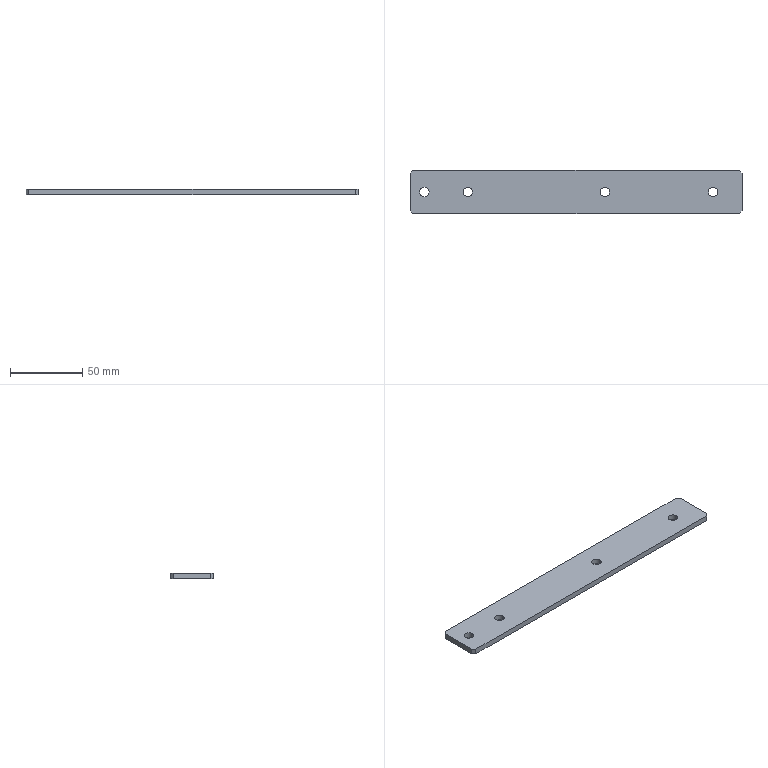Part | SolidWorks | features Chamfer 1, Extrusion 1 | 1 solid | 18 faces | box 230 x 30 x 4 mm | volume 27037 mm3 | plane 10 | cylinder 8 | commonest cylinder face diameters 6.5 x8
STEP:
#1=CARTESIAN_POINT('',(91.75,0.,4.));
#2=VERTEX_POINT('',#1);
#3=CARTESIAN_POINT('',(98.25,0.,4.));
#4=VERTEX_POINT('',#3);
#5=CARTESIAN_POINT('',(95.,0.,4.));
#6=DIRECTION('',(0.,0.,1.));
#7=DIRECTION('',(1.,0.,0.));
#8=AXIS2_PLACEMENT_3D('',#5,#6,#7);
#9=CIRCLE('',#8,3.25);
#10=EDGE_CURVE('',#2,#4,#9,.T.);
#11=ORIENTED_EDGE('',*,*,#10,.T.);
#12=CARTESIAN_POINT('',(98.25,0.,0.));
#13=VERTEX_POINT('',#12);
#14=CARTESIAN_POINT('',(98.25,0.,4.));
#15=DIRECTION('',(0.,0.,-1.));
#16=VECTOR('',#15,1000.);
#17=LINE('',#14,#16);
#18=EDGE_CURVE('',#4,#13,#17,.T.);
#19=ORIENTED_EDGE('',*,*,#18,.T.);
#20=CARTESIAN_POINT('',(91.75,0.,0.));
#21=VERTEX_POINT('',#20);
#22=CARTESIAN_POINT('',(95.,0.,0.));
#23=DIRECTION('',(0.,0.,1.));
#24=DIRECTION('',(1.,0.,0.));
#25=AXIS2_PLACEMENT_3D('',#22,#23,#24);
#26=CIRCLE('',#25,3.25);
#27=EDGE_CURVE('',#21,#13,#26,.T.);
#28=ORIENTED_EDGE('',*,*,#27,.F.);
#29=CARTESIAN_POINT('',(91.75,0.,4.));
#30=DIRECTION('',(0.,0.,-1.));
#31=VECTOR('',#30,1000.);
#32=LINE('',#29,#31);
#33=EDGE_CURVE('',#2,#21,#32,.T.);
#34=ORIENTED_EDGE('',*,*,#33,.F.);
#35=EDGE_LOOP('',(#11,#19,#28,#34));
#36=FACE_OUTER_BOUND('',#35,.T.);
#37=CARTESIAN_POINT('',(95.,0.,4.));
#38=DIRECTION('',(0.,0.,-1.));
#39=DIRECTION('',(-1.,0.,0.));
#40=AXIS2_PLACEMENT_3D('',#37,#38,#39);
#41=CYLINDRICAL_SURFACE('',#40,3.25);
#42=ADVANCED_FACE('',(#36),#41,.F.);
#43=CARTESIAN_POINT('',(16.75,0.,4.));
#44=VERTEX_POINT('',#43);
#45=CARTESIAN_POINT('',(23.25,0.,4.));
#46=VERTEX_POINT('',#45);
#47=CARTESIAN_POINT('',(20.,0.,4.));
#48=DIRECTION('',(0.,0.,1.));
#49=DIRECTION('',(1.,0.,0.));
#50=AXIS2_PLACEMENT_3D('',#47,#48,#49);
#51=CIRCLE('',#50,3.25);
#52=EDGE_CURVE('',#44,#46,#51,.T.);
#53=ORIENTED_EDGE('',*,*,#52,.T.);
#54=CARTESIAN_POINT('',(23.25,0.,0.));
#55=VERTEX_POINT('',#54);
#56=CARTESIAN_POINT('',(23.25,0.,4.));
#57=DIRECTION('',(0.,0.,-1.));
#58=VECTOR('',#57,1000.);
#59=LINE('',#56,#58);
#60=EDGE_CURVE('',#46,#55,#59,.T.);
#61=ORIENTED_EDGE('',*,*,#60,.T.);
#62=CARTESIAN_POINT('',(16.75,0.,0.));
#63=VERTEX_POINT('',#62);
#64=CARTESIAN_POINT('',(20.,0.,0.));
#65=DIRECTION('',(0.,0.,1.));
#66=DIRECTION('',(1.,0.,0.));
#67=AXIS2_PLACEMENT_3D('',#64,#65,#66);
#68=CIRCLE('',#67,3.25);
#69=EDGE_CURVE('',#63,#55,#68,.T.);
#70=ORIENTED_EDGE('',*,*,#69,.F.);
#71=CARTESIAN_POINT('',(16.75,0.,4.));
#72=DIRECTION('',(0.,0.,-1.));
#73=VECTOR('',#72,1000.);
#74=LINE('',#71,#73);
#75=EDGE_CURVE('',#44,#63,#74,.T.);
#76=ORIENTED_EDGE('',*,*,#75,.F.);
#77=EDGE_LOOP('',(#53,#61,#70,#76));
#78=FACE_OUTER_BOUND('',#77,.T.);
#79=CARTESIAN_POINT('',(20.,0.,4.));
#80=DIRECTION('',(0.,0.,-1.));
#81=DIRECTION('',(-1.,0.,0.));
#82=AXIS2_PLACEMENT_3D('',#79,#80,#81);
#83=CYLINDRICAL_SURFACE('',#82,3.25);
#84=ADVANCED_FACE('',(#78),#83,.F.);
#85=CARTESIAN_POINT('',(-78.25,0.,4.));
#86=VERTEX_POINT('',#85);
#87=CARTESIAN_POINT('',(-71.75,0.,4.));
#88=VERTEX_POINT('',#87);
#89=CARTESIAN_POINT('',(-75.,0.,4.));
#90=DIRECTION('',(0.,0.,1.));
#91=DIRECTION('',(1.,0.,0.));
#92=AXIS2_PLACEMENT_3D('',#89,#90,#91);
#93=CIRCLE('',#92,3.25);
#94=EDGE_CURVE('',#86,#88,#93,.T.);
#95=ORIENTED_EDGE('',*,*,#94,.T.);
#96=CARTESIAN_POINT('',(-71.75,0.,0.));
#97=VERTEX_POINT('',#96);
#98=CARTESIAN_POINT('',(-71.75,0.,4.));
#99=DIRECTION('',(0.,0.,-1.));
#100=VECTOR('',#99,1000.);
#101=LINE('',#98,#100);
#102=EDGE_CURVE('',#88,#97,#101,.T.);
#103=ORIENTED_EDGE('',*,*,#102,.T.);
#104=CARTESIAN_POINT('',(-78.25,0.,0.));
#105=VERTEX_POINT('',#104);
#106=CARTESIAN_POINT('',(-75.,0.,0.));
#107=DIRECTION('',(0.,0.,1.));
#108=DIRECTION('',(1.,0.,0.));
#109=AXIS2_PLACEMENT_3D('',#106,#107,#108);
#110=CIRCLE('',#109,3.25);
#111=EDGE_CURVE('',#105,#97,#110,.T.);
#112=ORIENTED_EDGE('',*,*,#111,.F.);
#113=CARTESIAN_POINT('',(-78.25,0.,4.));
#114=DIRECTION('',(0.,0.,-1.));
#115=VECTOR('',#114,1000.);
#116=LINE('',#113,#115);
#117=EDGE_CURVE('',#86,#105,#116,.T.);
#118=ORIENTED_EDGE('',*,*,#117,.F.);
#119=EDGE_LOOP('',(#95,#103,#112,#118));
#120=FACE_OUTER_BOUND('',#119,.T.);
#121=CARTESIAN_POINT('',(-75.,0.,4.));
#122=DIRECTION('',(0.,0.,-1.));
#123=DIRECTION('',(-1.,0.,0.));
#124=AXIS2_PLACEMENT_3D('',#121,#122,#123);
#125=CYLINDRICAL_SURFACE('',#124,3.25);
#126=ADVANCED_FACE('',(#120),#125,.F.);
#127=CARTESIAN_POINT('',(-108.25,0.,4.));
#128=VERTEX_POINT('',#127);
#129=CARTESIAN_POINT('',(-101.75,0.,4.));
#130=VERTEX_POINT('',#129);
#131=CARTESIAN_POINT('',(-105.,0.,4.));
#132=DIRECTION('',(0.,0.,1.));
#133=DIRECTION('',(1.,0.,0.));
#134=AXIS2_PLACEMENT_3D('',#131,#132,#133);
#135=CIRCLE('',#134,3.25);
#136=EDGE_CURVE('',#128,#130,#135,.T.);
#137=ORIENTED_EDGE('',*,*,#136,.T.);
#138=CARTESIAN_POINT('',(-101.75,0.,0.));
#139=VERTEX_POINT('',#138);
#140=CARTESIAN_POINT('',(-101.75,0.,4.));
#141=DIRECTION('',(0.,0.,-1.));
#142=VECTOR('',#141,1000.);
#143=LINE('',#140,#142);
#144=EDGE_CURVE('',#130,#139,#143,.T.);
#145=ORIENTED_EDGE('',*,*,#144,.T.);
#146=CARTESIAN_POINT('',(-108.25,0.,0.));
#147=VERTEX_POINT('',#146);
#148=CARTESIAN_POINT('',(-105.,0.,0.));
#149=DIRECTION('',(0.,0.,1.));
#150=DIRECTION('',(1.,0.,0.));
#151=AXIS2_PLACEMENT_3D('',#148,#149,#150);
#152=CIRCLE('',#151,3.25);
#153=EDGE_CURVE('',#147,#139,#152,.T.);
#154=ORIENTED_EDGE('',*,*,#153,.F.);
#155=CARTESIAN_POINT('',(-108.25,0.,4.));
#156=DIRECTION('',(0.,0.,-1.));
#157=VECTOR('',#156,1000.);
#158=LINE('',#155,#157);
#159=EDGE_CURVE('',#128,#147,#158,.T.);
#160=ORIENTED_EDGE('',*,*,#159,.F.);
#161=EDGE_LOOP('',(#137,#145,#154,#160));
#162=FACE_OUTER_BOUND('',#161,.T.);
#163=CARTESIAN_POINT('',(-105.,0.,4.));
#164=DIRECTION('',(0.,0.,-1.));
#165=DIRECTION('',(-1.,0.,0.));
#166=AXIS2_PLACEMENT_3D('',#163,#164,#165);
#167=CYLINDRICAL_SURFACE('',#166,3.25);
#168=ADVANCED_FACE('',(#162),#167,.F.);
#169=CARTESIAN_POINT('',(-115.,13.,4.));
#170=VERTEX_POINT('',#169);
#171=CARTESIAN_POINT('',(-115.,-13.,4.));
#172=VERTEX_POINT('',#171);
#173=CARTESIAN_POINT('',(-115.,15.,4.));
#174=DIRECTION('',(0.,-1.,0.));
#175=VECTOR('',#174,1000.);
#176=LINE('',#173,#175);
#177=EDGE_CURVE('',#170,#172,#176,.T.);
#178=ORIENTED_EDGE('',*,*,#177,.T.);
#179=CARTESIAN_POINT('',(-113.,-15.,4.));
#180=VERTEX_POINT('',#179);
#181=CARTESIAN_POINT('',(-113.,-15.,4.));
#182=DIRECTION('',(0.7071,-0.7071,0.));
#183=VECTOR('',#182,1000.);
#184=LINE('',#181,#183);
#185=EDGE_CURVE('',#172,#180,#184,.T.);
#186=ORIENTED_EDGE('',*,*,#185,.T.);
#187=CARTESIAN_POINT('',(113.,-15.,4.));
#188=VERTEX_POINT('',#187);
#189=CARTESIAN_POINT('',(115.,-15.,4.));
#190=DIRECTION('',(1.,0.,0.));
#191=VECTOR('',#190,1000.);
#192=LINE('',#189,#191);
#193=EDGE_CURVE('',#180,#188,#192,.T.);
#194=ORIENTED_EDGE('',*,*,#193,.T.);
#195=CARTESIAN_POINT('',(115.,-13.,4.));
#196=VERTEX_POINT('',#195);
#197=CARTESIAN_POINT('',(115.,-13.,4.));
#198=DIRECTION('',(0.7071,0.7071,0.));
#199=VECTOR('',#198,1000.);
#200=LINE('',#197,#199);
#201=EDGE_CURVE('',#188,#196,#200,.T.);
#202=ORIENTED_EDGE('',*,*,#201,.T.);
#203=CARTESIAN_POINT('',(115.,13.,4.));
#204=VERTEX_POINT('',#203);
#205=CARTESIAN_POINT('',(115.,15.,4.));
#206=DIRECTION('',(0.,1.,0.));
#207=VECTOR('',#206,1000.);
#208=LINE('',#205,#207);
#209=EDGE_CURVE('',#196,#204,#208,.T.);
#210=ORIENTED_EDGE('',*,*,#209,.T.);
#211=CARTESIAN_POINT('',(113.,15.,4.));
#212=VERTEX_POINT('',#211);
#213=CARTESIAN_POINT('',(113.,15.,4.));
#214=DIRECTION('',(-0.7071,0.7071,0.));
#215=VECTOR('',#214,1000.);
#216=LINE('',#213,#215);
#217=EDGE_CURVE('',#204,#212,#216,.T.);
#218=ORIENTED_EDGE('',*,*,#217,.T.);
#219=CARTESIAN_POINT('',(-113.,15.,4.));
#220=VERTEX_POINT('',#219);
#221=CARTESIAN_POINT('',(115.,15.,4.));
#222=DIRECTION('',(-1.,0.,0.));
#223=VECTOR('',#222,1000.);
#224=LINE('',#221,#223);
#225=EDGE_CURVE('',#212,#220,#224,.T.);
#226=ORIENTED_EDGE('',*,*,#225,.T.);
#227=CARTESIAN_POINT('',(-115.,13.,4.));
#228=DIRECTION('',(-0.7071,-0.7071,0.));
#229=VECTOR('',#228,1000.);
#230=LINE('',#227,#229);
#231=EDGE_CURVE('',#220,#170,#230,.T.);
#232=ORIENTED_EDGE('',*,*,#231,.T.);
#233=EDGE_LOOP('',(#178,#186,#194,#202,#210,#218,#226,#232));
#234=FACE_OUTER_BOUND('',#233,.T.);
#235=ORIENTED_EDGE('',*,*,#136,.F.);
#236=CARTESIAN_POINT('',(-105.,0.,4.));
#237=DIRECTION('',(0.,0.,1.));
#238=DIRECTION('',(1.,0.,0.));
#239=AXIS2_PLACEMENT_3D('',#236,#237,#238);
#240=CIRCLE('',#239,3.25);
#241=EDGE_CURVE('',#130,#128,#240,.T.);
#242=ORIENTED_EDGE('',*,*,#241,.F.);
#243=EDGE_LOOP('',(#235,#242));
#244=FACE_BOUND('',#243,.T.);
#245=ORIENTED_EDGE('',*,*,#94,.F.);
#246=CARTESIAN_POINT('',(-75.,0.,4.));
#247=DIRECTION('',(0.,0.,1.));
#248=DIRECTION('',(1.,0.,0.));
#249=AXIS2_PLACEMENT_3D('',#246,#247,#248);
#250=CIRCLE('',#249,3.25);
#251=EDGE_CURVE('',#88,#86,#250,.T.);
#252=ORIENTED_EDGE('',*,*,#251,.F.);
#253=EDGE_LOOP('',(#245,#252));
#254=FACE_BOUND('',#253,.T.);
#255=ORIENTED_EDGE('',*,*,#52,.F.);
#256=CARTESIAN_POINT('',(20.,0.,4.));
#257=DIRECTION('',(0.,0.,1.));
#258=DIRECTION('',(1.,0.,0.));
#259=AXIS2_PLACEMENT_3D('',#256,#257,#258);
#260=CIRCLE('',#259,3.25);
#261=EDGE_CURVE('',#46,#44,#260,.T.);
#262=ORIENTED_EDGE('',*,*,#261,.F.);
#263=EDGE_LOOP('',(#255,#262));
#264=FACE_BOUND('',#263,.T.);
#265=ORIENTED_EDGE('',*,*,#10,.F.);
#266=CARTESIAN_POINT('',(95.,0.,4.));
#267=DIRECTION('',(0.,0.,1.));
#268=DIRECTION('',(1.,0.,0.));
#269=AXIS2_PLACEMENT_3D('',#266,#267,#268);
#270=CIRCLE('',#269,3.25);
#271=EDGE_CURVE('',#4,#2,#270,.T.);
#272=ORIENTED_EDGE('',*,*,#271,.F.);
#273=EDGE_LOOP('',(#265,#272));
#274=FACE_BOUND('',#273,.T.);
#275=CARTESIAN_POINT('',(0.,0.,4.));
#276=DIRECTION('',(0.,0.,-1.));
#277=DIRECTION('',(-1.,0.,0.));
#278=AXIS2_PLACEMENT_3D('',#275,#276,#277);
#279=PLANE('',#278);
#280=ADVANCED_FACE('',(#234,#244,#254,#264,#274),#279,.F.);
#281=ORIENTED_EDGE('',*,*,#69,.T.);
#282=CARTESIAN_POINT('',(20.,0.,0.));
#283=DIRECTION('',(0.,0.,1.));
#284=DIRECTION('',(1.,0.,0.));
#285=AXIS2_PLACEMENT_3D('',#282,#283,#284);
#286=CIRCLE('',#285,3.25);
#287=EDGE_CURVE('',#55,#63,#286,.T.);
#288=ORIENTED_EDGE('',*,*,#287,.T.);
#289=EDGE_LOOP('',(#281,#288));
#290=FACE_BOUND('',#289,.T.);
#291=ORIENTED_EDGE('',*,*,#153,.T.);
#292=CARTESIAN_POINT('',(-105.,0.,0.));
#293=DIRECTION('',(0.,0.,1.));
#294=DIRECTION('',(1.,0.,0.));
#295=AXIS2_PLACEMENT_3D('',#292,#293,#294);
#296=CIRCLE('',#295,3.25);
#297=EDGE_CURVE('',#139,#147,#296,.T.);
#298=ORIENTED_EDGE('',*,*,#297,.T.);
#299=EDGE_LOOP('',(#291,#298));
#300=FACE_BOUND('',#299,.T.);
#301=CARTESIAN_POINT('',(-113.,-15.,0.));
#302=VERTEX_POINT('',#301);
#303=CARTESIAN_POINT('',(113.,-15.,0.));
#304=VERTEX_POINT('',#303);
#305=CARTESIAN_POINT('',(115.,-15.,0.));
#306=DIRECTION('',(1.,0.,0.));
#307=VECTOR('',#306,1000.);
#308=LINE('',#305,#307);
#309=EDGE_CURVE('',#302,#304,#308,.T.);
#310=ORIENTED_EDGE('',*,*,#309,.F.);
#311=CARTESIAN_POINT('',(-115.,-13.,0.));
#312=VERTEX_POINT('',#311);
#313=CARTESIAN_POINT('',(-64.,-64.,0.));
#314=DIRECTION('',(-0.7071,0.7071,0.));
#315=VECTOR('',#314,1000.);
#316=LINE('',#313,#315);
#317=EDGE_CURVE('',#302,#312,#316,.T.);
#318=ORIENTED_EDGE('',*,*,#317,.T.);
#319=CARTESIAN_POINT('',(-115.,13.,0.));
#320=VERTEX_POINT('',#319);
#321=CARTESIAN_POINT('',(-115.,15.,0.));
#322=DIRECTION('',(0.,-1.,0.));
#323=VECTOR('',#322,1000.);
#324=LINE('',#321,#323);
#325=EDGE_CURVE('',#320,#312,#324,.T.);
#326=ORIENTED_EDGE('',*,*,#325,.F.);
#327=CARTESIAN_POINT('',(-113.,15.,0.));
#328=VERTEX_POINT('',#327);
#329=CARTESIAN_POINT('',(-64.,64.,0.));
#330=DIRECTION('',(0.7071,0.7071,0.));
#331=VECTOR('',#330,1000.);
#332=LINE('',#329,#331);
#333=EDGE_CURVE('',#320,#328,#332,.T.);
#334=ORIENTED_EDGE('',*,*,#333,.T.);
#335=CARTESIAN_POINT('',(113.,15.,0.));
#336=VERTEX_POINT('',#335);
#337=CARTESIAN_POINT('',(115.,15.,0.));
#338=DIRECTION('',(-1.,0.,0.));
#339=VECTOR('',#338,1000.);
#340=LINE('',#337,#339);
#341=EDGE_CURVE('',#336,#328,#340,.T.);
#342=ORIENTED_EDGE('',*,*,#341,.F.);
#343=CARTESIAN_POINT('',(115.,13.,0.));
#344=VERTEX_POINT('',#343);
#345=CARTESIAN_POINT('',(64.,64.,0.));
#346=DIRECTION('',(0.7071,-0.7071,0.));
#347=VECTOR('',#346,1000.);
#348=LINE('',#345,#347);
#349=EDGE_CURVE('',#336,#344,#348,.T.);
#350=ORIENTED_EDGE('',*,*,#349,.T.);
#351=CARTESIAN_POINT('',(115.,-13.,0.));
#352=VERTEX_POINT('',#351);
#353=CARTESIAN_POINT('',(115.,15.,0.));
#354=DIRECTION('',(0.,1.,0.));
#355=VECTOR('',#354,1000.);
#356=LINE('',#353,#355);
#357=EDGE_CURVE('',#352,#344,#356,.T.);
#358=ORIENTED_EDGE('',*,*,#357,.F.);
#359=CARTESIAN_POINT('',(64.,-64.,0.));
#360=DIRECTION('',(-0.7071,-0.7071,0.));
#361=VECTOR('',#360,1000.);
#362=LINE('',#359,#361);
#363=EDGE_CURVE('',#352,#304,#362,.T.);
#364=ORIENTED_EDGE('',*,*,#363,.T.);
#365=EDGE_LOOP('',(#310,#318,#326,#334,#342,#350,#358,#364));
#366=FACE_OUTER_BOUND('',#365,.T.);
#367=ORIENTED_EDGE('',*,*,#111,.T.);
#368=CARTESIAN_POINT('',(-75.,0.,0.));
#369=DIRECTION('',(0.,0.,1.));
#370=DIRECTION('',(1.,0.,0.));
#371=AXIS2_PLACEMENT_3D('',#368,#369,#370);
#372=CIRCLE('',#371,3.25);
#373=EDGE_CURVE('',#97,#105,#372,.T.);
#374=ORIENTED_EDGE('',*,*,#373,.T.);
#375=EDGE_LOOP('',(#367,#374));
#376=FACE_BOUND('',#375,.T.);
#377=ORIENTED_EDGE('',*,*,#27,.T.);
#378=CARTESIAN_POINT('',(95.,0.,0.));
#379=DIRECTION('',(0.,0.,1.));
#380=DIRECTION('',(1.,0.,0.));
#381=AXIS2_PLACEMENT_3D('',#378,#379,#380);
#382=CIRCLE('',#381,3.25);
#383=EDGE_CURVE('',#13,#21,#382,.T.);
#384=ORIENTED_EDGE('',*,*,#383,.T.);
#385=EDGE_LOOP('',(#377,#384));
#386=FACE_BOUND('',#385,.T.);
#387=CARTESIAN_POINT('',(0.,0.,0.));
#388=DIRECTION('',(0.,0.,-1.));
#389=DIRECTION('',(-1.,0.,0.));
#390=AXIS2_PLACEMENT_3D('',#387,#388,#389);
#391=PLANE('',#390);
#392=ADVANCED_FACE('',(#290,#300,#366,#376,#386),#391,.T.);
#393=ORIENTED_EDGE('',*,*,#325,.T.);
#394=CARTESIAN_POINT('',(-115.,-13.,4.));
#395=DIRECTION('',(0.,0.,1.));
#396=VECTOR('',#395,1000.);
#397=LINE('',#394,#396);
#398=EDGE_CURVE('',#312,#172,#397,.T.);
#399=ORIENTED_EDGE('',*,*,#398,.T.);
#400=ORIENTED_EDGE('',*,*,#177,.F.);
#401=CARTESIAN_POINT('',(-115.,13.,4.));
#402=DIRECTION('',(0.,0.,-1.));
#403=VECTOR('',#402,1000.);
#404=LINE('',#401,#403);
#405=EDGE_CURVE('',#170,#320,#404,.T.);
#406=ORIENTED_EDGE('',*,*,#405,.T.);
#407=EDGE_LOOP('',(#393,#399,#400,#406));
#408=FACE_OUTER_BOUND('',#407,.T.);
#409=CARTESIAN_POINT('',(-115.,15.,4.));
#410=DIRECTION('',(1.,0.,0.));
#411=DIRECTION('',(0.,0.,-1.));
#412=AXIS2_PLACEMENT_3D('',#409,#410,#411);
#413=PLANE('',#412);
#414=ADVANCED_FACE('',(#408),#413,.F.);
#415=ORIENTED_EDGE('',*,*,#193,.F.);
#416=CARTESIAN_POINT('',(-113.,-15.,4.));
#417=DIRECTION('',(0.,0.,-1.));
#418=VECTOR('',#417,1000.);
#419=LINE('',#416,#418);
#420=EDGE_CURVE('',#180,#302,#419,.T.);
#421=ORIENTED_EDGE('',*,*,#420,.T.);
#422=ORIENTED_EDGE('',*,*,#309,.T.);
#423=CARTESIAN_POINT('',(113.,-15.,4.));
#424=DIRECTION('',(0.,0.,1.));
#425=VECTOR('',#424,1000.);
#426=LINE('',#423,#425);
#427=EDGE_CURVE('',#304,#188,#426,.T.);
#428=ORIENTED_EDGE('',*,*,#427,.T.);
#429=EDGE_LOOP('',(#415,#421,#422,#428));
#430=FACE_OUTER_BOUND('',#429,.T.);
#431=CARTESIAN_POINT('',(115.,-15.,4.));
#432=DIRECTION('',(0.,1.,0.));
#433=DIRECTION('',(-1.,0.,0.));
#434=AXIS2_PLACEMENT_3D('',#431,#432,#433);
#435=PLANE('',#434);
#436=ADVANCED_FACE('',(#430),#435,.F.);
#437=ORIENTED_EDGE('',*,*,#209,.F.);
#438=CARTESIAN_POINT('',(115.,-13.,4.));
#439=DIRECTION('',(0.,0.,-1.));
#440=VECTOR('',#439,1000.);
#441=LINE('',#438,#440);
#442=EDGE_CURVE('',#196,#352,#441,.T.);
#443=ORIENTED_EDGE('',*,*,#442,.T.);
#444=ORIENTED_EDGE('',*,*,#357,.T.);
#445=CARTESIAN_POINT('',(115.,13.,4.));
#446=DIRECTION('',(0.,0.,1.));
#447=VECTOR('',#446,1000.);
#448=LINE('',#445,#447);
#449=EDGE_CURVE('',#344,#204,#448,.T.);
#450=ORIENTED_EDGE('',*,*,#449,.T.);
#451=EDGE_LOOP('',(#437,#443,#444,#450));
#452=FACE_OUTER_BOUND('',#451,.T.);
#453=CARTESIAN_POINT('',(115.,15.,4.));
#454=DIRECTION('',(-1.,0.,0.));
#455=DIRECTION('',(0.,-1.,0.));
#456=AXIS2_PLACEMENT_3D('',#453,#454,#455);
#457=PLANE('',#456);
#458=ADVANCED_FACE('',(#452),#457,.F.);
#459=ORIENTED_EDGE('',*,*,#341,.T.);
#460=CARTESIAN_POINT('',(-113.,15.,4.));
#461=DIRECTION('',(0.,0.,1.));
#462=VECTOR('',#461,1000.);
#463=LINE('',#460,#462);
#464=EDGE_CURVE('',#328,#220,#463,.T.);
#465=ORIENTED_EDGE('',*,*,#464,.T.);
#466=ORIENTED_EDGE('',*,*,#225,.F.);
#467=CARTESIAN_POINT('',(113.,15.,4.));
#468=DIRECTION('',(0.,0.,-1.));
#469=VECTOR('',#468,1000.);
#470=LINE('',#467,#469);
#471=EDGE_CURVE('',#212,#336,#470,.T.);
#472=ORIENTED_EDGE('',*,*,#471,.T.);
#473=EDGE_LOOP('',(#459,#465,#466,#472));
#474=FACE_OUTER_BOUND('',#473,.T.);
#475=CARTESIAN_POINT('',(115.,15.,4.));
#476=DIRECTION('',(0.,-1.,0.));
#477=DIRECTION('',(1.,0.,0.));
#478=AXIS2_PLACEMENT_3D('',#475,#476,#477);
#479=PLANE('',#478);
#480=ADVANCED_FACE('',(#474),#479,.F.);
#481=ORIENTED_EDGE('',*,*,#144,.F.);
#482=ORIENTED_EDGE('',*,*,#241,.T.);
#483=ORIENTED_EDGE('',*,*,#159,.T.);
#484=ORIENTED_EDGE('',*,*,#297,.F.);
#485=EDGE_LOOP('',(#481,#482,#483,#484));
#486=FACE_OUTER_BOUND('',#485,.T.);
#487=CARTESIAN_POINT('',(-105.,0.,4.));
#488=DIRECTION('',(0.,0.,-1.));
#489=DIRECTION('',(-1.,0.,0.));
#490=AXIS2_PLACEMENT_3D('',#487,#488,#489);
#491=CYLINDRICAL_SURFACE('',#490,3.25);
#492=ADVANCED_FACE('',(#486),#491,.F.);
#493=ORIENTED_EDGE('',*,*,#102,.F.);
#494=ORIENTED_EDGE('',*,*,#251,.T.);
#495=ORIENTED_EDGE('',*,*,#117,.T.);
#496=ORIENTED_EDGE('',*,*,#373,.F.);
#497=EDGE_LOOP('',(#493,#494,#495,#496));
#498=FACE_OUTER_BOUND('',#497,.T.);
#499=CARTESIAN_POINT('',(-75.,0.,4.));
#500=DIRECTION('',(0.,0.,-1.));
#501=DIRECTION('',(-1.,0.,0.));
#502=AXIS2_PLACEMENT_3D('',#499,#500,#501);
#503=CYLINDRICAL_SURFACE('',#502,3.25);
#504=ADVANCED_FACE('',(#498),#503,.F.);
#505=ORIENTED_EDGE('',*,*,#60,.F.);
#506=ORIENTED_EDGE('',*,*,#261,.T.);
#507=ORIENTED_EDGE('',*,*,#75,.T.);
#508=ORIENTED_EDGE('',*,*,#287,.F.);
#509=EDGE_LOOP('',(#505,#506,#507,#508));
#510=FACE_OUTER_BOUND('',#509,.T.);
#511=CARTESIAN_POINT('',(20.,0.,4.));
#512=DIRECTION('',(0.,0.,-1.));
#513=DIRECTION('',(-1.,0.,0.));
#514=AXIS2_PLACEMENT_3D('',#511,#512,#513);
#515=CYLINDRICAL_SURFACE('',#514,3.25);
#516=ADVANCED_FACE('',(#510),#515,.F.);
#517=ORIENTED_EDGE('',*,*,#18,.F.);
#518=ORIENTED_EDGE('',*,*,#271,.T.);
#519=ORIENTED_EDGE('',*,*,#33,.T.);
#520=ORIENTED_EDGE('',*,*,#383,.F.);
#521=EDGE_LOOP('',(#517,#518,#519,#520));
#522=FACE_OUTER_BOUND('',#521,.T.);
#523=CARTESIAN_POINT('',(95.,0.,4.));
#524=DIRECTION('',(0.,0.,-1.));
#525=DIRECTION('',(-1.,0.,0.));
#526=AXIS2_PLACEMENT_3D('',#523,#524,#525);
#527=CYLINDRICAL_SURFACE('',#526,3.25);
#528=ADVANCED_FACE('',(#522),#527,.F.);
#529=ORIENTED_EDGE('',*,*,#185,.F.);
#530=ORIENTED_EDGE('',*,*,#398,.F.);
#531=ORIENTED_EDGE('',*,*,#317,.F.);
#532=ORIENTED_EDGE('',*,*,#420,.F.);
#533=EDGE_LOOP('',(#529,#530,#531,#532));
#534=FACE_OUTER_BOUND('',#533,.T.);
#535=CARTESIAN_POINT('',(-113.,-15.,4.));
#536=DIRECTION('',(0.7071,0.7071,0.));
#537=DIRECTION('',(0.,0.,-1.));
#538=AXIS2_PLACEMENT_3D('',#535,#536,#537);
#539=PLANE('',#538);
#540=ADVANCED_FACE('',(#534),#539,.F.);
#541=ORIENTED_EDGE('',*,*,#231,.F.);
#542=ORIENTED_EDGE('',*,*,#464,.F.);
#543=ORIENTED_EDGE('',*,*,#333,.F.);
#544=ORIENTED_EDGE('',*,*,#405,.F.);
#545=EDGE_LOOP('',(#541,#542,#543,#544));
#546=FACE_OUTER_BOUND('',#545,.T.);
#547=CARTESIAN_POINT('',(-115.,13.,4.));
#548=DIRECTION('',(0.7071,-0.7071,0.));
#549=DIRECTION('',(0.,0.,-1.));
#550=AXIS2_PLACEMENT_3D('',#547,#548,#549);
#551=PLANE('',#550);
#552=ADVANCED_FACE('',(#546),#551,.F.);
#553=ORIENTED_EDGE('',*,*,#201,.F.);
#554=ORIENTED_EDGE('',*,*,#427,.F.);
#555=ORIENTED_EDGE('',*,*,#363,.F.);
#556=ORIENTED_EDGE('',*,*,#442,.F.);
#557=EDGE_LOOP('',(#553,#554,#555,#556));
#558=FACE_OUTER_BOUND('',#557,.T.);
#559=CARTESIAN_POINT('',(115.,-13.,4.));
#560=DIRECTION('',(-0.7071,0.7071,0.));
#561=DIRECTION('',(0.,0.,-1.));
#562=AXIS2_PLACEMENT_3D('',#559,#560,#561);
#563=PLANE('',#562);
#564=ADVANCED_FACE('',(#558),#563,.F.);
#565=ORIENTED_EDGE('',*,*,#217,.F.);
#566=ORIENTED_EDGE('',*,*,#449,.F.);
#567=ORIENTED_EDGE('',*,*,#349,.F.);
#568=ORIENTED_EDGE('',*,*,#471,.F.);
#569=EDGE_LOOP('',(#565,#566,#567,#568));
#570=FACE_OUTER_BOUND('',#569,.T.);
#571=CARTESIAN_POINT('',(113.,15.,4.));
#572=DIRECTION('',(-0.7071,-0.7071,0.));
#573=DIRECTION('',(0.,0.,-1.));
#574=AXIS2_PLACEMENT_3D('',#571,#572,#573);
#575=PLANE('',#574);
#576=ADVANCED_FACE('',(#570),#575,.F.);
#577=CLOSED_SHELL('',(#42,#84,#126,#168,#280,#392,#414,#436,#458,#480,#492,#504,#516,#528,#540,#552,#564,#576));
#578=MANIFOLD_SOLID_BREP('',#577);
#579=CARTESIAN_POINT('',(0.,0.,0.));
#580=DIRECTION('',(0.,0.,1.));
#581=DIRECTION('',(1.,0.,0.));
#582=AXIS2_PLACEMENT_3D('',#579,#580,#581);
#583=(LENGTH_UNIT()NAMED_UNIT(*)SI_UNIT(.MILLI.,.METRE.));
#584=UNCERTAINTY_MEASURE_WITH_UNIT(LENGTH_MEASURE(0.00001),#583,'','');
#585=(NAMED_UNIT(*)PLANE_ANGLE_UNIT()SI_UNIT($,.RADIAN.));
#586=(NAMED_UNIT(*)SI_UNIT($,.STERADIAN.)SOLID_ANGLE_UNIT());
#587=(GEOMETRIC_REPRESENTATION_CONTEXT(3)GLOBAL_UNCERTAINTY_ASSIGNED_CONTEXT((#584))GLOBAL_UNIT_ASSIGNED_CONTEXT((#583,#585,#586))REPRESENTATION_CONTEXT('',''));
#588=ADVANCED_BREP_SHAPE_REPRESENTATION('',(#578,#582),#587);